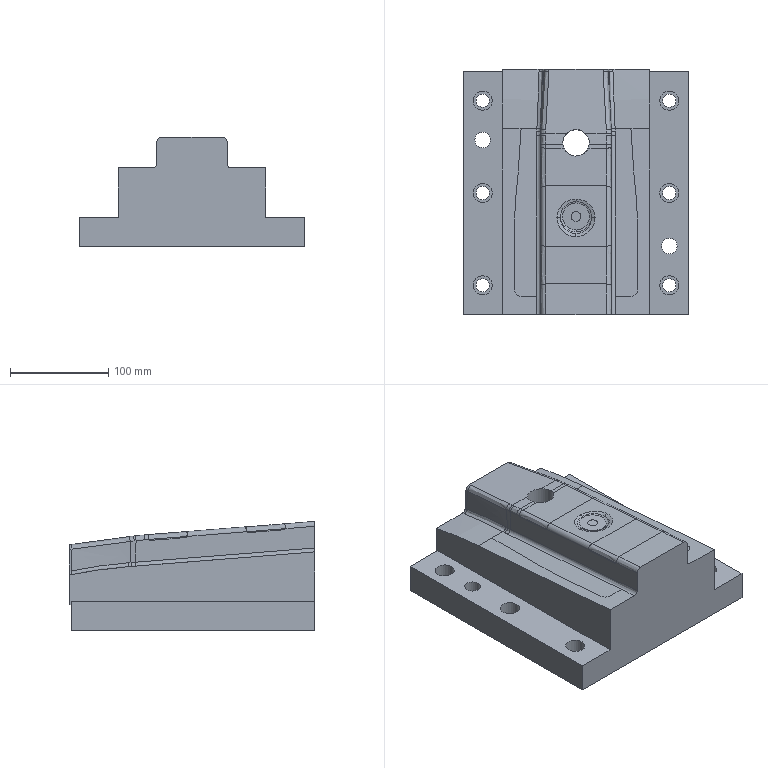Part | NX | features solid 2 | 1 solid | 104 faces | box 230 x 250 x 111.173 mm | volume 3625709 mm3 | spline 68 | plane 19 | cylinder 17 | commonest cylinder face diameters 13.5 x6 19.5 x6 16 x2 20 x2 27 x1